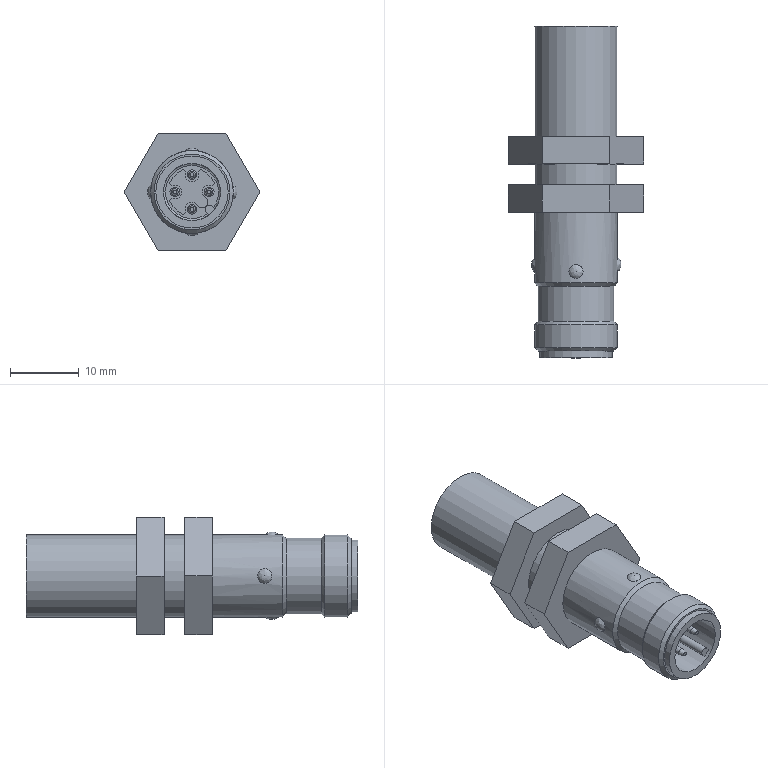Part | STEP file | 1 solid | 158 faces | box 19.63 x 48.1 x 17 mm | volume 5552 mm3 | cylinder 72 | plane 58 | cone 17 | torus 7 | spline 4 | commonest cylinder face diameters 2 x15 0.6 x14 1 x8 7 x7 0.8 x4 1.3 x4